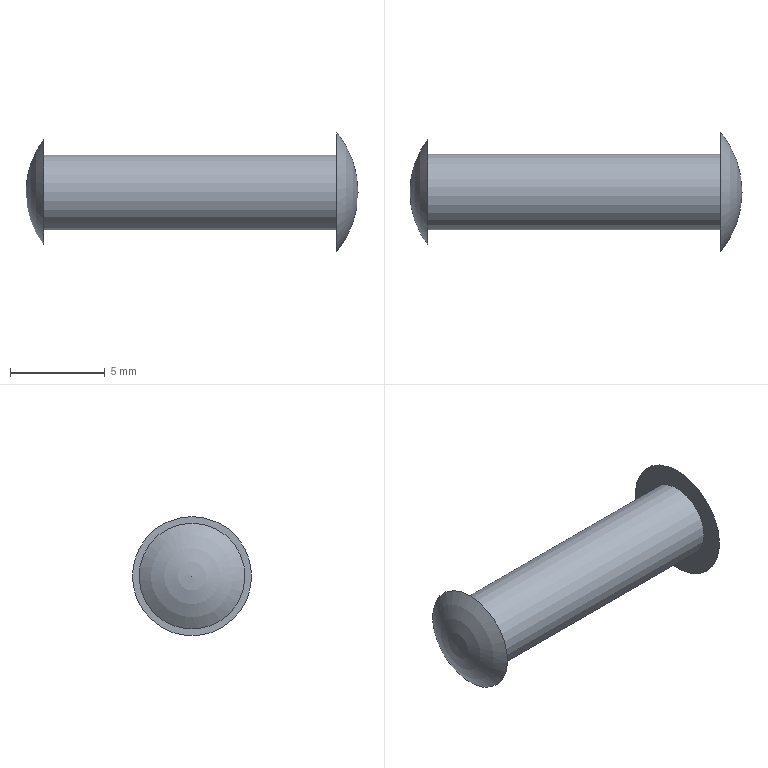Part | STEP file | 1-64 | 1 solid | 5 faces | box 17.557 x 6.3 x 6.3 mm | volume 224.928 mm3 | plane 2 | sphere 2 | cylinder 1 | commonest cylinder face diameters 4 x1
STEP:
#1=CARTESIAN_POINT('',(0.,0.,0.));
#2=DIRECTION('',(0.,0.,1.));
#3=DIRECTION('',(1.,0.,0.));
#4=AXIS2_PLACEMENT_3D('',#1,#2,#3);
#5=CARTESIAN_POINT('',(0.,2.,0.));
#6=VERTEX_POINT('',#5);
#7=CARTESIAN_POINT('',(0.,0.,0.));
#8=DIRECTION('',(1.,0.,0.));
#9=DIRECTION('',(0.,1.,0.));
#10=AXIS2_PLACEMENT_3D('',#7,#8,#9);
#11=CIRCLE('',#10,2.);
#12=CARTESIAN_POINT('',(0.,0.,0.));
#13=DIRECTION('',(1.,0.,0.));
#14=DIRECTION('',(0.,1.,0.));
#15=AXIS2_PLACEMENT_3D('',#12,#13,#14);
#16=CYLINDRICAL_SURFACE('',#15,2.);
#17=CARTESIAN_POINT('',(0.,0.));
#18=DIRECTION('',(1.,0.));
#19=VECTOR('',#18,1.);
#20=LINE('',#17,#19);
#21=(GEOMETRIC_REPRESENTATION_CONTEXT(2)PARAMETRIC_REPRESENTATION_CONTEXT()REPRESENTATION_CONTEXT('',''));
#22=DEFINITIONAL_REPRESENTATION('',(#20),#21);
#23=PCURVE('',#16,#22);
#24=CARTESIAN_POINT('',(0.,0.,0.));
#25=DIRECTION('',(1.,0.,0.));
#26=DIRECTION('',(0.,0.,1.));
#27=AXIS2_PLACEMENT_3D('',#24,#25,#26);
#28=PLANE('',#27);
#29=CARTESIAN_POINT('',(0.,0.));
#30=DIRECTION('',(0.,-1.));
#31=AXIS2_PLACEMENT_2D('',#29,#30);
#32=CIRCLE('',#31,2.);
#33=(GEOMETRIC_REPRESENTATION_CONTEXT(2)PARAMETRIC_REPRESENTATION_CONTEXT()REPRESENTATION_CONTEXT('',''));
#34=DEFINITIONAL_REPRESENTATION('',(#32),#33);
#35=PCURVE('',#28,#34);
#36=SURFACE_CURVE('',#11,(#23,#35),.PCURVE_S1.);
#37=EDGE_CURVE('',#6,#6,#36,.T.);
#38=ORIENTED_EDGE('',*,*,#37,.T.);
#39=CARTESIAN_POINT('',(15.5,2.,0.));
#40=VERTEX_POINT('',#39);
#41=CARTESIAN_POINT('',(0.,2.,0.));
#42=DIRECTION('',(1.,0.,0.));
#43=VECTOR('',#42,1.);
#44=LINE('',#41,#43);
#45=CARTESIAN_POINT('',(6.283,0.));
#46=DIRECTION('',(0.,1.));
#47=VECTOR('',#46,1.);
#48=LINE('',#45,#47);
#49=(GEOMETRIC_REPRESENTATION_CONTEXT(2)PARAMETRIC_REPRESENTATION_CONTEXT()REPRESENTATION_CONTEXT('',''));
#50=DEFINITIONAL_REPRESENTATION('',(#48),#49);
#51=PCURVE('',#16,#50);
#52=CARTESIAN_POINT('',(0.,0.));
#53=DIRECTION('',(0.,1.));
#54=VECTOR('',#53,1.);
#55=LINE('',#52,#54);
#56=(GEOMETRIC_REPRESENTATION_CONTEXT(2)PARAMETRIC_REPRESENTATION_CONTEXT()REPRESENTATION_CONTEXT('',''));
#57=DEFINITIONAL_REPRESENTATION('',(#55),#56);
#58=PCURVE('',#16,#57);
#59=SEAM_CURVE('',#44,(#51,#58),.PCURVE_S1.);
#60=EDGE_CURVE('',#6,#40,#59,.T.);
#61=ORIENTED_EDGE('',*,*,#60,.T.);
#62=CARTESIAN_POINT('',(15.5,0.,0.));
#63=DIRECTION('',(1.,0.,0.));
#64=DIRECTION('',(0.,1.,0.));
#65=AXIS2_PLACEMENT_3D('',#62,#63,#64);
#66=CIRCLE('',#65,2.);
#67=CARTESIAN_POINT('',(0.,15.5));
#68=DIRECTION('',(1.,0.));
#69=VECTOR('',#68,1.);
#70=LINE('',#67,#69);
#71=(GEOMETRIC_REPRESENTATION_CONTEXT(2)PARAMETRIC_REPRESENTATION_CONTEXT()REPRESENTATION_CONTEXT('',''));
#72=DEFINITIONAL_REPRESENTATION('',(#70),#71);
#73=PCURVE('',#16,#72);
#74=CARTESIAN_POINT('',(15.5,0.,0.));
#75=DIRECTION('',(-1.,0.,0.));
#76=DIRECTION('',(0.,0.,1.));
#77=AXIS2_PLACEMENT_3D('',#74,#75,#76);
#78=PLANE('',#77);
#79=CARTESIAN_POINT('',(0.,2.));
#80=CARTESIAN_POINT('',(3.464,2.));
#81=CARTESIAN_POINT('',(1.732,-1.));
#82=CARTESIAN_POINT('',(0.,-4.));
#83=CARTESIAN_POINT('',(-1.732,-1.));
#84=CARTESIAN_POINT('',(-3.464,2.));
#85=CARTESIAN_POINT('',(0.,2.));
#86=(BOUNDED_CURVE()B_SPLINE_CURVE(2,(#79,#80,#81,#82,#83,#84,#85),.UNSPECIFIED.,.T.,.F.)B_SPLINE_CURVE_WITH_KNOTS((1,2,2,2,2,1),(-2.094,0.,2.094,4.189,6.283,8.378),.UNSPECIFIED.)CURVE()GEOMETRIC_REPRESENTATION_ITEM()RATIONAL_B_SPLINE_CURVE((1.,0.5,1.,0.5,1.,0.5,1.))REPRESENTATION_ITEM(''));
#87=(GEOMETRIC_REPRESENTATION_CONTEXT(2)PARAMETRIC_REPRESENTATION_CONTEXT()REPRESENTATION_CONTEXT('',''));
#88=DEFINITIONAL_REPRESENTATION('',(#86),#87);
#89=PCURVE('',#78,#88);
#90=SURFACE_CURVE('',#66,(#73,#89),.PCURVE_S1.);
#91=EDGE_CURVE('',#40,#40,#90,.T.);
#92=ORIENTED_EDGE('',*,*,#91,.F.);
#93=ORIENTED_EDGE('',*,*,#60,.F.);
#94=EDGE_LOOP('',(#38,#61,#92,#93));
#95=FACE_BOUND('',#94,.T.);
#96=ADVANCED_FACE('',(#95),#16,.T.);
#97=CARTESIAN_POINT('',(0.,0.,2.8));
#98=VERTEX_POINT('',#97);
#99=CARTESIAN_POINT('',(0.,0.,0.));
#100=DIRECTION('',(1.,0.,0.));
#101=DIRECTION('',(0.,0.,1.));
#102=AXIS2_PLACEMENT_3D('',#99,#100,#101);
#103=CIRCLE('',#102,2.8);
#104=CARTESIAN_POINT('',(0.,0.));
#105=DIRECTION('',(1.,0.));
#106=AXIS2_PLACEMENT_2D('',#104,#105);
#107=CIRCLE('',#106,2.8);
#108=(GEOMETRIC_REPRESENTATION_CONTEXT(2)PARAMETRIC_REPRESENTATION_CONTEXT()REPRESENTATION_CONTEXT('',''));
#109=DEFINITIONAL_REPRESENTATION('',(#107),#108);
#110=PCURVE('',#28,#109);
#111=CARTESIAN_POINT('',(3.701,0.,0.));
#112=DIRECTION('',(1.,0.,0.));
#113=DIRECTION('',(0.,0.,1.));
#114=AXIS2_PLACEMENT_3D('',#111,#112,#113);
#115=SPHERICAL_SURFACE('',#114,4.641);
#116=CARTESIAN_POINT('',(0.,-0.9231));
#117=CARTESIAN_POINT('',(0.0952,-0.9231));
#118=CARTESIAN_POINT('',(0.2856,-0.9231));
#119=CARTESIAN_POINT('',(0.5712,-0.9231));
#120=CARTESIAN_POINT('',(0.8568,-0.9231));
#121=CARTESIAN_POINT('',(1.142,-0.9231));
#122=CARTESIAN_POINT('',(1.428,-0.9231));
#123=CARTESIAN_POINT('',(1.714,-0.9231));
#124=CARTESIAN_POINT('',(1.999,-0.9231));
#125=CARTESIAN_POINT('',(2.285,-0.9231));
#126=CARTESIAN_POINT('',(2.57,-0.9231));
#127=CARTESIAN_POINT('',(2.856,-0.9231));
#128=CARTESIAN_POINT('',(3.142,-0.9231));
#129=CARTESIAN_POINT('',(3.427,-0.9231));
#130=CARTESIAN_POINT('',(3.713,-0.9231));
#131=CARTESIAN_POINT('',(3.998,-0.9231));
#132=CARTESIAN_POINT('',(4.284,-0.9231));
#133=CARTESIAN_POINT('',(4.57,-0.9231));
#134=CARTESIAN_POINT('',(4.855,-0.9231));
#135=CARTESIAN_POINT('',(5.141,-0.9231));
#136=CARTESIAN_POINT('',(5.426,-0.9231));
#137=CARTESIAN_POINT('',(5.712,-0.9231));
#138=CARTESIAN_POINT('',(5.998,-0.9231));
#139=CARTESIAN_POINT('',(6.188,-0.9231));
#140=CARTESIAN_POINT('',(6.283,-0.9231));
#141=B_SPLINE_CURVE_WITH_KNOTS('',3,(#116,#117,#118,#119,#120,#121,#122,#123,#124,#125,#126,#127,#128,#129,#130,#131,#132,#133,#134,#135,#136,#137,#138,#139,#140),.UNSPECIFIED.,.F.,.F.,(4,1,1,1,1,1,1,1,1,1,1,1,1,1,1,1,1,1,1,1,1,1,4),(0.,0.2856,0.5712,0.8568,1.142,1.428,1.714,1.999,2.285,2.57,2.856,3.142,3.427,3.713,3.998,4.284,4.57,4.855,5.141,5.426,5.712,5.998,6.283),.QUASI_UNIFORM_KNOTS.);
#142=(GEOMETRIC_REPRESENTATION_CONTEXT(2)PARAMETRIC_REPRESENTATION_CONTEXT()REPRESENTATION_CONTEXT('',''));
#143=DEFINITIONAL_REPRESENTATION('',(#141),#142);
#144=PCURVE('',#115,#143);
#145=SURFACE_CURVE('',#103,(#110,#144),.PCURVE_S1.);
#146=EDGE_CURVE('',#98,#98,#145,.T.);
#147=ORIENTED_EDGE('',*,*,#146,.T.);
#148=EDGE_LOOP('',(#147));
#149=FACE_BOUND('',#148,.T.);
#150=ORIENTED_EDGE('',*,*,#37,.F.);
#151=EDGE_LOOP('',(#150));
#152=FACE_BOUND('',#151,.T.);
#153=ADVANCED_FACE('',(#149,#152),#28,.T.);
#154=CARTESIAN_POINT('',(15.5,0.,3.15));
#155=VERTEX_POINT('',#154);
#156=CARTESIAN_POINT('',(15.5,0.,0.));
#157=DIRECTION('',(1.,0.,0.));
#158=DIRECTION('',(0.,0.,1.));
#159=AXIS2_PLACEMENT_3D('',#156,#157,#158);
#160=CIRCLE('',#159,3.15);
#161=CARTESIAN_POINT('',(3.15,0.));
#162=CARTESIAN_POINT('',(3.15,-5.456));
#163=CARTESIAN_POINT('',(-1.575,-2.728));
#164=CARTESIAN_POINT('',(-6.3,0.));
#165=CARTESIAN_POINT('',(-1.575,2.728));
#166=CARTESIAN_POINT('',(3.15,5.456));
#167=CARTESIAN_POINT('',(3.15,0.));
#168=(BOUNDED_CURVE()B_SPLINE_CURVE(2,(#161,#162,#163,#164,#165,#166,#167),.UNSPECIFIED.,.T.,.F.)B_SPLINE_CURVE_WITH_KNOTS((1,2,2,2,2,1),(-2.094,0.,2.094,4.189,6.283,8.378),.UNSPECIFIED.)CURVE()GEOMETRIC_REPRESENTATION_ITEM()RATIONAL_B_SPLINE_CURVE((1.,0.5,1.,0.5,1.,0.5,1.))REPRESENTATION_ITEM(''));
#169=(GEOMETRIC_REPRESENTATION_CONTEXT(2)PARAMETRIC_REPRESENTATION_CONTEXT()REPRESENTATION_CONTEXT('',''));
#170=DEFINITIONAL_REPRESENTATION('',(#168),#169);
#171=PCURVE('',#78,#170);
#172=CARTESIAN_POINT('',(11.617,0.,0.));
#173=DIRECTION('',(1.,0.,0.));
#174=DIRECTION('',(0.,0.,1.));
#175=AXIS2_PLACEMENT_3D('',#172,#173,#174);
#176=SPHERICAL_SURFACE('',#175,5.);
#177=CARTESIAN_POINT('',(0.,0.8892));
#178=CARTESIAN_POINT('',(0.0952,0.8892));
#179=CARTESIAN_POINT('',(0.2856,0.8892));
#180=CARTESIAN_POINT('',(0.5712,0.8892));
#181=CARTESIAN_POINT('',(0.8568,0.8892));
#182=CARTESIAN_POINT('',(1.142,0.8892));
#183=CARTESIAN_POINT('',(1.428,0.8892));
#184=CARTESIAN_POINT('',(1.714,0.8892));
#185=CARTESIAN_POINT('',(1.999,0.8892));
#186=CARTESIAN_POINT('',(2.285,0.8892));
#187=CARTESIAN_POINT('',(2.57,0.8892));
#188=CARTESIAN_POINT('',(2.856,0.8892));
#189=CARTESIAN_POINT('',(3.142,0.8892));
#190=CARTESIAN_POINT('',(3.427,0.8892));
#191=CARTESIAN_POINT('',(3.713,0.8892));
#192=CARTESIAN_POINT('',(3.998,0.8892));
#193=CARTESIAN_POINT('',(4.284,0.8892));
#194=CARTESIAN_POINT('',(4.57,0.8892));
#195=CARTESIAN_POINT('',(4.855,0.8892));
#196=CARTESIAN_POINT('',(5.141,0.8892));
#197=CARTESIAN_POINT('',(5.426,0.8892));
#198=CARTESIAN_POINT('',(5.712,0.8892));
#199=CARTESIAN_POINT('',(5.998,0.8892));
#200=CARTESIAN_POINT('',(6.188,0.8892));
#201=CARTESIAN_POINT('',(6.283,0.8892));
#202=B_SPLINE_CURVE_WITH_KNOTS('',3,(#177,#178,#179,#180,#181,#182,#183,#184,#185,#186,#187,#188,#189,#190,#191,#192,#193,#194,#195,#196,#197,#198,#199,#200,#201),.UNSPECIFIED.,.F.,.F.,(4,1,1,1,1,1,1,1,1,1,1,1,1,1,1,1,1,1,1,1,1,1,4),(0.,0.2856,0.5712,0.8568,1.142,1.428,1.714,1.999,2.285,2.57,2.856,3.142,3.427,3.713,3.998,4.284,4.57,4.855,5.141,5.426,5.712,5.998,6.283),.QUASI_UNIFORM_KNOTS.);
#203=(GEOMETRIC_REPRESENTATION_CONTEXT(2)PARAMETRIC_REPRESENTATION_CONTEXT()REPRESENTATION_CONTEXT('',''));
#204=DEFINITIONAL_REPRESENTATION('',(#202),#203);
#205=PCURVE('',#176,#204);
#206=SURFACE_CURVE('',#160,(#171,#205),.PCURVE_S1.);
#207=EDGE_CURVE('',#155,#155,#206,.T.);
#208=ORIENTED_EDGE('',*,*,#207,.F.);
#209=EDGE_LOOP('',(#208));
#210=FACE_BOUND('',#209,.T.);
#211=ORIENTED_EDGE('',*,*,#91,.T.);
#212=EDGE_LOOP('',(#211));
#213=FACE_BOUND('',#212,.T.);
#214=ADVANCED_FACE('',(#210,#213),#78,.T.);
#215=CARTESIAN_POINT('',(-0.9398,0.,0.));
#216=VERTEX_POINT('',#215);
#217=CARTESIAN_POINT('',(3.701,0.,0.));
#218=DIRECTION('',(0.,-1.,0.));
#219=DIRECTION('',(-0.7975,0.,0.6033));
#220=AXIS2_PLACEMENT_3D('',#217,#218,#219);
#221=CIRCLE('',#220,4.641);
#222=CARTESIAN_POINT('',(0.,-0.9231));
#223=CARTESIAN_POINT('',(0.,-0.9329));
#224=CARTESIAN_POINT('',(0.,-0.9526));
#225=CARTESIAN_POINT('',(0.,-0.982));
#226=CARTESIAN_POINT('',(0.,-1.011));
#227=CARTESIAN_POINT('',(0.,-1.041));
#228=CARTESIAN_POINT('',(0.,-1.07));
#229=CARTESIAN_POINT('',(0.,-1.1));
#230=CARTESIAN_POINT('',(0.,-1.129));
#231=CARTESIAN_POINT('',(0.,-1.159));
#232=CARTESIAN_POINT('',(0.,-1.188));
#233=CARTESIAN_POINT('',(0.,-1.218));
#234=CARTESIAN_POINT('',(0.,-1.247));
#235=CARTESIAN_POINT('',(0.,-1.276));
#236=CARTESIAN_POINT('',(0.,-1.306));
#237=CARTESIAN_POINT('',(0.,-1.335));
#238=CARTESIAN_POINT('',(0.,-1.365));
#239=CARTESIAN_POINT('',(0.,-1.394));
#240=CARTESIAN_POINT('',(0.,-1.424));
#241=CARTESIAN_POINT('',(0.,-1.453));
#242=CARTESIAN_POINT('',(0.,-1.482));
#243=CARTESIAN_POINT('',(0.,-1.512));
#244=CARTESIAN_POINT('',(0.,-1.541));
#245=CARTESIAN_POINT('',(0.,-1.561));
#246=CARTESIAN_POINT('',(0.,-1.571));
#247=B_SPLINE_CURVE_WITH_KNOTS('',3,(#222,#223,#224,#225,#226,#227,#228,#229,#230,#231,#232,#233,#234,#235,#236,#237,#238,#239,#240,#241,#242,#243,#244,#245,#246),.UNSPECIFIED.,.F.,.F.,(4,1,1,1,1,1,1,1,1,1,1,1,1,1,1,1,1,1,1,1,1,1,4),(0.,0.02944,0.05888,0.08832,0.1178,0.1472,0.1766,0.2061,0.2355,0.265,0.2944,0.3238,0.3533,0.3827,0.4122,0.4416,0.471,0.5005,0.5299,0.5594,0.5888,0.6182,0.6477),.QUASI_UNIFORM_KNOTS.);
#248=(GEOMETRIC_REPRESENTATION_CONTEXT(2)PARAMETRIC_REPRESENTATION_CONTEXT()REPRESENTATION_CONTEXT('',''));
#249=DEFINITIONAL_REPRESENTATION('',(#247),#248);
#250=PCURVE('',#115,#249);
#251=CARTESIAN_POINT('',(6.283,-0.9231));
#252=CARTESIAN_POINT('',(6.283,-0.9329));
#253=CARTESIAN_POINT('',(6.283,-0.9526));
#254=CARTESIAN_POINT('',(6.283,-0.982));
#255=CARTESIAN_POINT('',(6.283,-1.011));
#256=CARTESIAN_POINT('',(6.283,-1.041));
#257=CARTESIAN_POINT('',(6.283,-1.07));
#258=CARTESIAN_POINT('',(6.283,-1.1));
#259=CARTESIAN_POINT('',(6.283,-1.129));
#260=CARTESIAN_POINT('',(6.283,-1.159));
#261=CARTESIAN_POINT('',(6.283,-1.188));
#262=CARTESIAN_POINT('',(6.283,-1.218));
#263=CARTESIAN_POINT('',(6.283,-1.247));
#264=CARTESIAN_POINT('',(6.283,-1.276));
#265=CARTESIAN_POINT('',(6.283,-1.306));
#266=CARTESIAN_POINT('',(6.283,-1.335));
#267=CARTESIAN_POINT('',(6.283,-1.365));
#268=CARTESIAN_POINT('',(6.283,-1.394));
#269=CARTESIAN_POINT('',(6.283,-1.424));
#270=CARTESIAN_POINT('',(6.283,-1.453));
#271=CARTESIAN_POINT('',(6.283,-1.482));
#272=CARTESIAN_POINT('',(6.283,-1.512));
#273=CARTESIAN_POINT('',(6.283,-1.541));
#274=CARTESIAN_POINT('',(6.283,-1.561));
#275=CARTESIAN_POINT('',(6.283,-1.571));
#276=B_SPLINE_CURVE_WITH_KNOTS('',3,(#251,#252,#253,#254,#255,#256,#257,#258,#259,#260,#261,#262,#263,#264,#265,#266,#267,#268,#269,#270,#271,#272,#273,#274,#275),.UNSPECIFIED.,.F.,.F.,(4,1,1,1,1,1,1,1,1,1,1,1,1,1,1,1,1,1,1,1,1,1,4),(0.,0.02944,0.05888,0.08832,0.1178,0.1472,0.1766,0.2061,0.2355,0.265,0.2944,0.3238,0.3533,0.3827,0.4122,0.4416,0.471,0.5005,0.5299,0.5594,0.5888,0.6182,0.6477),.QUASI_UNIFORM_KNOTS.);
#277=(GEOMETRIC_REPRESENTATION_CONTEXT(2)PARAMETRIC_REPRESENTATION_CONTEXT()REPRESENTATION_CONTEXT('',''));
#278=DEFINITIONAL_REPRESENTATION('',(#276),#277);
#279=PCURVE('',#115,#278);
#280=SEAM_CURVE('',#221,(#250,#279),.PCURVE_S1.);
#281=EDGE_CURVE('',#98,#216,#280,.T.);
#282=ORIENTED_EDGE('',*,*,#281,.T.);
#283=ORIENTED_EDGE('',*,*,#281,.F.);
#284=ORIENTED_EDGE('',*,*,#146,.F.);
#285=EDGE_LOOP('',(#282,#283,#284));
#286=FACE_BOUND('',#285,.T.);
#287=ADVANCED_FACE('',(#286),#115,.T.);
#288=CARTESIAN_POINT('',(16.617,0.,0.));
#289=VERTEX_POINT('',#288);
#290=CARTESIAN_POINT('',(11.617,0.,0.));
#291=DIRECTION('',(0.,-1.,0.));
#292=DIRECTION('',(1.,0.,0.));
#293=AXIS2_PLACEMENT_3D('',#290,#291,#292);
#294=CIRCLE('',#293,5.);
#295=CARTESIAN_POINT('',(0.,1.571));
#296=CARTESIAN_POINT('',(0.,1.56));
#297=CARTESIAN_POINT('',(0.,1.54));
#298=CARTESIAN_POINT('',(0.,1.509));
#299=CARTESIAN_POINT('',(0.,1.478));
#300=CARTESIAN_POINT('',(0.,1.447));
#301=CARTESIAN_POINT('',(0.,1.416));
#302=CARTESIAN_POINT('',(0.,1.385));
#303=CARTESIAN_POINT('',(0.,1.354));
#304=CARTESIAN_POINT('',(0.,1.323));
#305=CARTESIAN_POINT('',(0.,1.292));
#306=CARTESIAN_POINT('',(0.,1.261));
#307=CARTESIAN_POINT('',(0.,1.23));
#308=CARTESIAN_POINT('',(0.,1.199));
#309=CARTESIAN_POINT('',(0.,1.168));
#310=CARTESIAN_POINT('',(0.,1.137));
#311=CARTESIAN_POINT('',(0.,1.106));
#312=CARTESIAN_POINT('',(0.,1.075));
#313=CARTESIAN_POINT('',(0.,1.044));
#314=CARTESIAN_POINT('',(0.,1.013));
#315=CARTESIAN_POINT('',(0.,0.9822));
#316=CARTESIAN_POINT('',(0.,0.9512));
#317=CARTESIAN_POINT('',(0.,0.9202));
#318=CARTESIAN_POINT('',(0.,0.8996));
#319=CARTESIAN_POINT('',(0.,0.8892));
#320=B_SPLINE_CURVE_WITH_KNOTS('',3,(#295,#296,#297,#298,#299,#300,#301,#302,#303,#304,#305,#306,#307,#308,#309,#310,#311,#312,#313,#314,#315,#316,#317,#318,#319),.UNSPECIFIED.,.F.,.F.,(4,1,1,1,1,1,1,1,1,1,1,1,1,1,1,1,1,1,1,1,1,1,4),(0.,0.03098,0.06196,0.09294,0.1239,0.1549,0.1859,0.2169,0.2478,0.2788,0.3098,0.3408,0.3718,0.4027,0.4337,0.4647,0.4957,0.5267,0.5576,0.5886,0.6196,0.6506,0.6816),.QUASI_UNIFORM_KNOTS.);
#321=(GEOMETRIC_REPRESENTATION_CONTEXT(2)PARAMETRIC_REPRESENTATION_CONTEXT()REPRESENTATION_CONTEXT('',''));
#322=DEFINITIONAL_REPRESENTATION('',(#320),#321);
#323=PCURVE('',#176,#322);
#324=CARTESIAN_POINT('',(6.283,1.571));
#325=CARTESIAN_POINT('',(6.283,1.56));
#326=CARTESIAN_POINT('',(6.283,1.54));
#327=CARTESIAN_POINT('',(6.283,1.509));
#328=CARTESIAN_POINT('',(6.283,1.478));
#329=CARTESIAN_POINT('',(6.283,1.447));
#330=CARTESIAN_POINT('',(6.283,1.416));
#331=CARTESIAN_POINT('',(6.283,1.385));
#332=CARTESIAN_POINT('',(6.283,1.354));
#333=CARTESIAN_POINT('',(6.283,1.323));
#334=CARTESIAN_POINT('',(6.283,1.292));
#335=CARTESIAN_POINT('',(6.283,1.261));
#336=CARTESIAN_POINT('',(6.283,1.23));
#337=CARTESIAN_POINT('',(6.283,1.199));
#338=CARTESIAN_POINT('',(6.283,1.168));
#339=CARTESIAN_POINT('',(6.283,1.137));
#340=CARTESIAN_POINT('',(6.283,1.106));
#341=CARTESIAN_POINT('',(6.283,1.075));
#342=CARTESIAN_POINT('',(6.283,1.044));
#343=CARTESIAN_POINT('',(6.283,1.013));
#344=CARTESIAN_POINT('',(6.283,0.9822));
#345=CARTESIAN_POINT('',(6.283,0.9512));
#346=CARTESIAN_POINT('',(6.283,0.9202));
#347=CARTESIAN_POINT('',(6.283,0.8996));
#348=CARTESIAN_POINT('',(6.283,0.8892));
#349=B_SPLINE_CURVE_WITH_KNOTS('',3,(#324,#325,#326,#327,#328,#329,#330,#331,#332,#333,#334,#335,#336,#337,#338,#339,#340,#341,#342,#343,#344,#345,#346,#347,#348),.UNSPECIFIED.,.F.,.F.,(4,1,1,1,1,1,1,1,1,1,1,1,1,1,1,1,1,1,1,1,1,1,4),(0.,0.03098,0.06196,0.09294,0.1239,0.1549,0.1859,0.2169,0.2478,0.2788,0.3098,0.3408,0.3718,0.4027,0.4337,0.4647,0.4957,0.5267,0.5576,0.5886,0.6196,0.6506,0.6816),.QUASI_UNIFORM_KNOTS.);
#350=(GEOMETRIC_REPRESENTATION_CONTEXT(2)PARAMETRIC_REPRESENTATION_CONTEXT()REPRESENTATION_CONTEXT('',''));
#351=DEFINITIONAL_REPRESENTATION('',(#349),#350);
#352=PCURVE('',#176,#351);
#353=SEAM_CURVE('',#294,(#323,#352),.PCURVE_S1.);
#354=EDGE_CURVE('',#289,#155,#353,.T.);
#355=ORIENTED_EDGE('',*,*,#354,.T.);
#356=ORIENTED_EDGE('',*,*,#207,.T.);
#357=ORIENTED_EDGE('',*,*,#354,.F.);
#358=EDGE_LOOP('',(#355,#356,#357));
#359=FACE_BOUND('',#358,.T.);
#360=ADVANCED_FACE('',(#359),#176,.T.);
#361=CLOSED_SHELL('',(#96,#153,#214,#287,#360));
#362=MANIFOLD_SOLID_BREP('',#361);
#363=(LENGTH_UNIT()NAMED_UNIT(*)SI_UNIT(.MILLI.,.METRE.));
#364=UNCERTAINTY_MEASURE_WITH_UNIT(LENGTH_MEASURE(0.0000001),#363,'','');
#365=(NAMED_UNIT(*)PLANE_ANGLE_UNIT()SI_UNIT($,.RADIAN.));
#366=(NAMED_UNIT(*)SI_UNIT($,.STERADIAN.)SOLID_ANGLE_UNIT());
#367=(GEOMETRIC_REPRESENTATION_CONTEXT(3)GLOBAL_UNCERTAINTY_ASSIGNED_CONTEXT((#364))GLOBAL_UNIT_ASSIGNED_CONTEXT((#363,#365,#366))REPRESENTATION_CONTEXT('',''));
#368=ADVANCED_BREP_SHAPE_REPRESENTATION('',(#4,#362),#367);